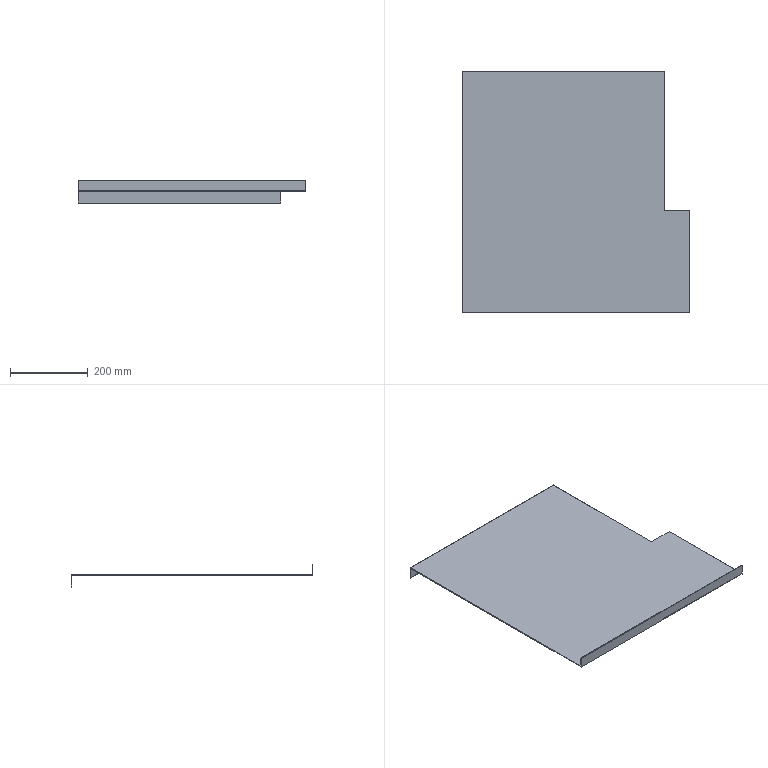Part | STEP file | 11-FG-JJ-01211 | 1 solid | 12 faces | box 586 x 623 x 57 mm | volume 744145 mm3 | plane 12
STEP:
#1=CARTESIAN_POINT('',(260.5,-46.737,0.));
#2=VERTEX_POINT('',#1);
#3=CARTESIAN_POINT('',(260.5,-46.737,2.));
#4=VERTEX_POINT('',#3);
#5=CARTESIAN_POINT('',(260.5,-46.737,0.));
#6=DIRECTION('',(0.,0.,1.));
#7=VECTOR('',#6,1000.);
#8=LINE('',#5,#7);
#9=EDGE_CURVE('',#2,#4,#8,.T.);
#10=ORIENTED_EDGE('',*,*,#9,.F.);
#11=CARTESIAN_POINT('',(260.5,309.5,0.));
#12=VERTEX_POINT('',#11);
#13=CARTESIAN_POINT('',(260.5,311.5,0.));
#14=DIRECTION('',(0.,1.,0.));
#15=VECTOR('',#14,1000.);
#16=LINE('',#13,#15);
#17=EDGE_CURVE('',#2,#12,#16,.T.);
#18=ORIENTED_EDGE('',*,*,#17,.T.);
#19=CARTESIAN_POINT('',(260.5,309.5,-30.));
#20=VERTEX_POINT('',#19);
#21=CARTESIAN_POINT('',(260.5,309.5,-30.));
#22=DIRECTION('',(0.,0.,1.));
#23=VECTOR('',#22,1000.);
#24=LINE('',#21,#23);
#25=EDGE_CURVE('',#20,#12,#24,.T.);
#26=ORIENTED_EDGE('',*,*,#25,.F.);
#27=CARTESIAN_POINT('',(260.5,311.5,-30.));
#28=VERTEX_POINT('',#27);
#29=CARTESIAN_POINT('',(260.5,311.5,-30.));
#30=DIRECTION('',(0.,-1.,0.));
#31=VECTOR('',#30,1000.);
#32=LINE('',#29,#31);
#33=EDGE_CURVE('',#28,#20,#32,.T.);
#34=ORIENTED_EDGE('',*,*,#33,.F.);
#35=CARTESIAN_POINT('',(260.5,311.5,2.));
#36=VERTEX_POINT('',#35);
#37=CARTESIAN_POINT('',(260.5,311.5,2.));
#38=DIRECTION('',(0.,0.,-1.));
#39=VECTOR('',#38,1000.);
#40=LINE('',#37,#39);
#41=EDGE_CURVE('',#36,#28,#40,.T.);
#42=ORIENTED_EDGE('',*,*,#41,.F.);
#43=CARTESIAN_POINT('',(260.5,311.5,2.));
#44=DIRECTION('',(0.,1.,0.));
#45=VECTOR('',#44,1000.);
#46=LINE('',#43,#45);
#47=EDGE_CURVE('',#4,#36,#46,.T.);
#48=ORIENTED_EDGE('',*,*,#47,.F.);
#49=EDGE_LOOP('',(#10,#18,#26,#34,#42,#48));
#50=FACE_OUTER_BOUND('',#49,.T.);
#51=CARTESIAN_POINT('',(260.5,311.5,2.));
#52=DIRECTION('',(-1.,0.,0.));
#53=DIRECTION('',(0.,-1.,0.));
#54=AXIS2_PLACEMENT_3D('',#51,#52,#53);
#55=PLANE('',#54);
#56=ADVANCED_FACE('',(#50),#55,.F.);
#57=CARTESIAN_POINT('',(-260.5,309.5,0.));
#58=VERTEX_POINT('',#57);
#59=CARTESIAN_POINT('',(260.5,309.5,0.));
#60=DIRECTION('',(-1.,0.,0.));
#61=VECTOR('',#60,1000.);
#62=LINE('',#59,#61);
#63=EDGE_CURVE('',#12,#58,#62,.T.);
#64=ORIENTED_EDGE('',*,*,#63,.F.);
#65=ORIENTED_EDGE('',*,*,#17,.F.);
#66=CARTESIAN_POINT('',(325.5,-46.737,0.));
#67=VERTEX_POINT('',#66);
#68=CARTESIAN_POINT('',(325.5,-46.737,0.));
#69=DIRECTION('',(-1.,0.,0.));
#70=VECTOR('',#69,1000.);
#71=LINE('',#68,#70);
#72=EDGE_CURVE('',#67,#2,#71,.T.);
#73=ORIENTED_EDGE('',*,*,#72,.F.);
#74=CARTESIAN_POINT('',(325.5,-311.5,0.));
#75=VERTEX_POINT('',#74);
#76=CARTESIAN_POINT('',(325.5,-46.737,0.));
#77=DIRECTION('',(0.,1.,0.));
#78=VECTOR('',#77,1000.);
#79=LINE('',#76,#78);
#80=EDGE_CURVE('',#75,#67,#79,.T.);
#81=ORIENTED_EDGE('',*,*,#80,.F.);
#82=CARTESIAN_POINT('',(-260.5,-311.5,0.));
#83=VERTEX_POINT('',#82);
#84=CARTESIAN_POINT('',(-260.5,-311.5,0.));
#85=DIRECTION('',(1.,0.,0.));
#86=VECTOR('',#85,1000.);
#87=LINE('',#84,#86);
#88=EDGE_CURVE('',#83,#75,#87,.T.);
#89=ORIENTED_EDGE('',*,*,#88,.F.);
#90=CARTESIAN_POINT('',(-260.5,311.5,0.));
#91=DIRECTION('',(0.,-1.,0.));
#92=VECTOR('',#91,1000.);
#93=LINE('',#90,#92);
#94=EDGE_CURVE('',#58,#83,#93,.T.);
#95=ORIENTED_EDGE('',*,*,#94,.F.);
#96=EDGE_LOOP('',(#64,#65,#73,#81,#89,#95));
#97=FACE_OUTER_BOUND('',#96,.T.);
#98=CARTESIAN_POINT('',(0.,0.,0.));
#99=DIRECTION('',(0.,0.,1.));
#100=DIRECTION('',(1.,0.,0.));
#101=AXIS2_PLACEMENT_3D('',#98,#99,#100);
#102=PLANE('',#101);
#103=ADVANCED_FACE('',(#97),#102,.F.);
#104=ORIENTED_EDGE('',*,*,#41,.T.);
#105=CARTESIAN_POINT('',(-260.5,311.5,-30.));
#106=VERTEX_POINT('',#105);
#107=CARTESIAN_POINT('',(260.5,311.5,-30.));
#108=DIRECTION('',(1.,0.,0.));
#109=VECTOR('',#108,1000.);
#110=LINE('',#107,#109);
#111=EDGE_CURVE('',#106,#28,#110,.T.);
#112=ORIENTED_EDGE('',*,*,#111,.F.);
#113=CARTESIAN_POINT('',(-260.5,311.5,2.));
#114=VERTEX_POINT('',#113);
#115=CARTESIAN_POINT('',(-260.5,311.5,2.));
#116=DIRECTION('',(0.,0.,-1.));
#117=VECTOR('',#116,1000.);
#118=LINE('',#115,#117);
#119=EDGE_CURVE('',#114,#106,#118,.T.);
#120=ORIENTED_EDGE('',*,*,#119,.F.);
#121=CARTESIAN_POINT('',(-260.5,311.5,2.));
#122=DIRECTION('',(-1.,0.,0.));
#123=VECTOR('',#122,1000.);
#124=LINE('',#121,#123);
#125=EDGE_CURVE('',#36,#114,#124,.T.);
#126=ORIENTED_EDGE('',*,*,#125,.F.);
#127=EDGE_LOOP('',(#104,#112,#120,#126));
#128=FACE_OUTER_BOUND('',#127,.T.);
#129=CARTESIAN_POINT('',(-260.5,311.5,2.));
#130=DIRECTION('',(0.,-1.,0.));
#131=DIRECTION('',(0.,0.,-1.));
#132=AXIS2_PLACEMENT_3D('',#129,#130,#131);
#133=PLANE('',#132);
#134=ADVANCED_FACE('',(#128),#133,.F.);
#135=ORIENTED_EDGE('',*,*,#119,.T.);
#136=CARTESIAN_POINT('',(-260.5,309.5,-30.));
#137=VERTEX_POINT('',#136);
#138=CARTESIAN_POINT('',(-260.5,311.5,-30.));
#139=DIRECTION('',(0.,1.,0.));
#140=VECTOR('',#139,1000.);
#141=LINE('',#138,#140);
#142=EDGE_CURVE('',#137,#106,#141,.T.);
#143=ORIENTED_EDGE('',*,*,#142,.F.);
#144=CARTESIAN_POINT('',(-260.5,309.5,-30.));
#145=DIRECTION('',(0.,0.,1.));
#146=VECTOR('',#145,1000.);
#147=LINE('',#144,#146);
#148=EDGE_CURVE('',#137,#58,#147,.T.);
#149=ORIENTED_EDGE('',*,*,#148,.T.);
#150=ORIENTED_EDGE('',*,*,#94,.T.);
#151=CARTESIAN_POINT('',(-260.5,-311.5,27.));
#152=VERTEX_POINT('',#151);
#153=CARTESIAN_POINT('',(-260.5,-311.5,2.));
#154=DIRECTION('',(0.,0.,-1.));
#155=VECTOR('',#154,1000.);
#156=LINE('',#153,#155);
#157=EDGE_CURVE('',#152,#83,#156,.T.);
#158=ORIENTED_EDGE('',*,*,#157,.F.);
#159=CARTESIAN_POINT('',(-260.5,-309.5,27.));
#160=VERTEX_POINT('',#159);
#161=CARTESIAN_POINT('',(-260.5,-311.5,27.));
#162=DIRECTION('',(0.,-1.,0.));
#163=VECTOR('',#162,1000.);
#164=LINE('',#161,#163);
#165=EDGE_CURVE('',#160,#152,#164,.T.);
#166=ORIENTED_EDGE('',*,*,#165,.F.);
#167=CARTESIAN_POINT('',(-260.5,-309.5,2.));
#168=VERTEX_POINT('',#167);
#169=CARTESIAN_POINT('',(-260.5,-309.5,27.));
#170=DIRECTION('',(0.,0.,-1.));
#171=VECTOR('',#170,1000.);
#172=LINE('',#169,#171);
#173=EDGE_CURVE('',#160,#168,#172,.T.);
#174=ORIENTED_EDGE('',*,*,#173,.T.);
#175=CARTESIAN_POINT('',(-260.5,311.5,2.));
#176=DIRECTION('',(0.,-1.,0.));
#177=VECTOR('',#176,1000.);
#178=LINE('',#175,#177);
#179=EDGE_CURVE('',#114,#168,#178,.T.);
#180=ORIENTED_EDGE('',*,*,#179,.F.);
#181=EDGE_LOOP('',(#135,#143,#149,#150,#158,#166,#174,#180));
#182=FACE_OUTER_BOUND('',#181,.T.);
#183=CARTESIAN_POINT('',(-260.5,311.5,2.));
#184=DIRECTION('',(1.,0.,0.));
#185=DIRECTION('',(0.,0.,-1.));
#186=AXIS2_PLACEMENT_3D('',#183,#184,#185);
#187=PLANE('',#186);
#188=ADVANCED_FACE('',(#182),#187,.F.);
#189=ORIENTED_EDGE('',*,*,#88,.T.);
#190=CARTESIAN_POINT('',(325.5,-311.5,27.));
#191=VERTEX_POINT('',#190);
#192=CARTESIAN_POINT('',(325.5,-311.5,0.));
#193=DIRECTION('',(0.,0.,-1.));
#194=VECTOR('',#193,1000.);
#195=LINE('',#192,#194);
#196=EDGE_CURVE('',#191,#75,#195,.T.);
#197=ORIENTED_EDGE('',*,*,#196,.F.);
#198=CARTESIAN_POINT('',(-260.5,-311.5,27.));
#199=DIRECTION('',(1.,0.,0.));
#200=VECTOR('',#199,1000.);
#201=LINE('',#198,#200);
#202=EDGE_CURVE('',#152,#191,#201,.T.);
#203=ORIENTED_EDGE('',*,*,#202,.F.);
#204=ORIENTED_EDGE('',*,*,#157,.T.);
#205=EDGE_LOOP('',(#189,#197,#203,#204));
#206=FACE_OUTER_BOUND('',#205,.T.);
#207=CARTESIAN_POINT('',(-260.5,-311.5,2.));
#208=DIRECTION('',(0.,1.,0.));
#209=DIRECTION('',(0.,0.,1.));
#210=AXIS2_PLACEMENT_3D('',#207,#208,#209);
#211=PLANE('',#210);
#212=ADVANCED_FACE('',(#206),#211,.F.);
#213=CARTESIAN_POINT('',(325.5,-309.5,2.));
#214=VERTEX_POINT('',#213);
#215=CARTESIAN_POINT('',(-260.5,-309.5,2.));
#216=DIRECTION('',(-1.,0.,0.));
#217=VECTOR('',#216,1000.);
#218=LINE('',#215,#217);
#219=EDGE_CURVE('',#214,#168,#218,.T.);
#220=ORIENTED_EDGE('',*,*,#219,.F.);
#221=CARTESIAN_POINT('',(325.5,-46.737,2.));
#222=VERTEX_POINT('',#221);
#223=CARTESIAN_POINT('',(325.5,-309.5,2.));
#224=DIRECTION('',(0.,-1.,0.));
#225=VECTOR('',#224,1000.);
#226=LINE('',#223,#225);
#227=EDGE_CURVE('',#222,#214,#226,.T.);
#228=ORIENTED_EDGE('',*,*,#227,.F.);
#229=CARTESIAN_POINT('',(325.5,-46.737,2.));
#230=DIRECTION('',(-1.,0.,0.));
#231=VECTOR('',#230,1000.);
#232=LINE('',#229,#231);
#233=EDGE_CURVE('',#222,#4,#232,.T.);
#234=ORIENTED_EDGE('',*,*,#233,.T.);
#235=ORIENTED_EDGE('',*,*,#47,.T.);
#236=ORIENTED_EDGE('',*,*,#125,.T.);
#237=ORIENTED_EDGE('',*,*,#179,.T.);
#238=EDGE_LOOP('',(#220,#228,#234,#235,#236,#237));
#239=FACE_OUTER_BOUND('',#238,.T.);
#240=CARTESIAN_POINT('',(0.,0.,2.));
#241=DIRECTION('',(0.,0.,1.));
#242=DIRECTION('',(1.,0.,0.));
#243=AXIS2_PLACEMENT_3D('',#240,#241,#242);
#244=PLANE('',#243);
#245=ADVANCED_FACE('',(#239),#244,.T.);
#246=ORIENTED_EDGE('',*,*,#63,.T.);
#247=ORIENTED_EDGE('',*,*,#148,.F.);
#248=CARTESIAN_POINT('',(260.5,309.5,-30.));
#249=DIRECTION('',(-1.,0.,0.));
#250=VECTOR('',#249,1000.);
#251=LINE('',#248,#250);
#252=EDGE_CURVE('',#20,#137,#251,.T.);
#253=ORIENTED_EDGE('',*,*,#252,.F.);
#254=ORIENTED_EDGE('',*,*,#25,.T.);
#255=EDGE_LOOP('',(#246,#247,#253,#254));
#256=FACE_OUTER_BOUND('',#255,.T.);
#257=CARTESIAN_POINT('',(260.5,309.5,-30.));
#258=DIRECTION('',(0.,1.,0.));
#259=DIRECTION('',(0.,0.,1.));
#260=AXIS2_PLACEMENT_3D('',#257,#258,#259);
#261=PLANE('',#260);
#262=ADVANCED_FACE('',(#256),#261,.F.);
#263=ORIENTED_EDGE('',*,*,#33,.T.);
#264=ORIENTED_EDGE('',*,*,#252,.T.);
#265=ORIENTED_EDGE('',*,*,#142,.T.);
#266=ORIENTED_EDGE('',*,*,#111,.T.);
#267=EDGE_LOOP('',(#263,#264,#265,#266));
#268=FACE_OUTER_BOUND('',#267,.T.);
#269=CARTESIAN_POINT('',(0.,0.,-30.));
#270=DIRECTION('',(0.,0.,-1.));
#271=DIRECTION('',(-1.,0.,0.));
#272=AXIS2_PLACEMENT_3D('',#269,#270,#271);
#273=PLANE('',#272);
#274=ADVANCED_FACE('',(#268),#273,.T.);
#275=ORIENTED_EDGE('',*,*,#219,.T.);
#276=ORIENTED_EDGE('',*,*,#173,.F.);
#277=CARTESIAN_POINT('',(325.5,-309.5,27.));
#278=VERTEX_POINT('',#277);
#279=CARTESIAN_POINT('',(-260.5,-309.5,27.));
#280=DIRECTION('',(-1.,0.,0.));
#281=VECTOR('',#280,1000.);
#282=LINE('',#279,#281);
#283=EDGE_CURVE('',#278,#160,#282,.T.);
#284=ORIENTED_EDGE('',*,*,#283,.F.);
#285=CARTESIAN_POINT('',(325.5,-309.5,2.));
#286=DIRECTION('',(0.,0.,1.));
#287=VECTOR('',#286,1000.);
#288=LINE('',#285,#287);
#289=EDGE_CURVE('',#214,#278,#288,.T.);
#290=ORIENTED_EDGE('',*,*,#289,.F.);
#291=EDGE_LOOP('',(#275,#276,#284,#290));
#292=FACE_OUTER_BOUND('',#291,.T.);
#293=CARTESIAN_POINT('',(-260.5,-309.5,27.));
#294=DIRECTION('',(0.,-1.,0.));
#295=DIRECTION('',(0.,0.,-1.));
#296=AXIS2_PLACEMENT_3D('',#293,#294,#295);
#297=PLANE('',#296);
#298=ADVANCED_FACE('',(#292),#297,.F.);
#299=ORIENTED_EDGE('',*,*,#165,.T.);
#300=ORIENTED_EDGE('',*,*,#202,.T.);
#301=CARTESIAN_POINT('',(325.5,-309.5,27.));
#302=DIRECTION('',(0.,-1.,0.));
#303=VECTOR('',#302,1000.);
#304=LINE('',#301,#303);
#305=EDGE_CURVE('',#278,#191,#304,.T.);
#306=ORIENTED_EDGE('',*,*,#305,.F.);
#307=ORIENTED_EDGE('',*,*,#283,.T.);
#308=EDGE_LOOP('',(#299,#300,#306,#307));
#309=FACE_OUTER_BOUND('',#308,.T.);
#310=CARTESIAN_POINT('',(0.,0.,27.));
#311=DIRECTION('',(0.,0.,-1.));
#312=DIRECTION('',(-1.,0.,0.));
#313=AXIS2_PLACEMENT_3D('',#310,#311,#312);
#314=PLANE('',#313);
#315=ADVANCED_FACE('',(#309),#314,.F.);
#316=ORIENTED_EDGE('',*,*,#9,.T.);
#317=ORIENTED_EDGE('',*,*,#233,.F.);
#318=CARTESIAN_POINT('',(325.5,-46.737,0.));
#319=DIRECTION('',(0.,0.,1.));
#320=VECTOR('',#319,1000.);
#321=LINE('',#318,#320);
#322=EDGE_CURVE('',#67,#222,#321,.T.);
#323=ORIENTED_EDGE('',*,*,#322,.F.);
#324=ORIENTED_EDGE('',*,*,#72,.T.);
#325=EDGE_LOOP('',(#316,#317,#323,#324));
#326=FACE_OUTER_BOUND('',#325,.T.);
#327=CARTESIAN_POINT('',(325.5,-46.737,0.));
#328=DIRECTION('',(0.,-1.,0.));
#329=DIRECTION('',(1.,0.,0.));
#330=AXIS2_PLACEMENT_3D('',#327,#328,#329);
#331=PLANE('',#330);
#332=ADVANCED_FACE('',(#326),#331,.F.);
#333=ORIENTED_EDGE('',*,*,#80,.T.);
#334=ORIENTED_EDGE('',*,*,#322,.T.);
#335=ORIENTED_EDGE('',*,*,#227,.T.);
#336=ORIENTED_EDGE('',*,*,#289,.T.);
#337=ORIENTED_EDGE('',*,*,#305,.T.);
#338=ORIENTED_EDGE('',*,*,#196,.T.);
#339=EDGE_LOOP('',(#333,#334,#335,#336,#337,#338));
#340=FACE_OUTER_BOUND('',#339,.T.);
#341=CARTESIAN_POINT('',(325.5,0.,0.));
#342=DIRECTION('',(-1.,0.,0.));
#343=DIRECTION('',(0.,-1.,0.));
#344=AXIS2_PLACEMENT_3D('',#341,#342,#343);
#345=PLANE('',#344);
#346=ADVANCED_FACE('',(#340),#345,.F.);
#347=CLOSED_SHELL('',(#56,#103,#134,#188,#212,#245,#262,#274,#298,#315,#332,#346));
#348=MANIFOLD_SOLID_BREP('',#347);
#349=CARTESIAN_POINT('',(0.,0.,0.));
#350=DIRECTION('',(0.,0.,1.));
#351=DIRECTION('',(1.,0.,0.));
#352=AXIS2_PLACEMENT_3D('',#349,#350,#351);
#353=(LENGTH_UNIT()NAMED_UNIT(*)SI_UNIT(.MILLI.,.METRE.));
#354=UNCERTAINTY_MEASURE_WITH_UNIT(LENGTH_MEASURE(0.00001),#353,'','');
#355=(NAMED_UNIT(*)PLANE_ANGLE_UNIT()SI_UNIT($,.RADIAN.));
#356=(NAMED_UNIT(*)SI_UNIT($,.STERADIAN.)SOLID_ANGLE_UNIT());
#357=(GEOMETRIC_REPRESENTATION_CONTEXT(3)GLOBAL_UNCERTAINTY_ASSIGNED_CONTEXT((#354))GLOBAL_UNIT_ASSIGNED_CONTEXT((#353,#355,#356))REPRESENTATION_CONTEXT('',''));
#358=ADVANCED_BREP_SHAPE_REPRESENTATION('',(#348,#352),#357);